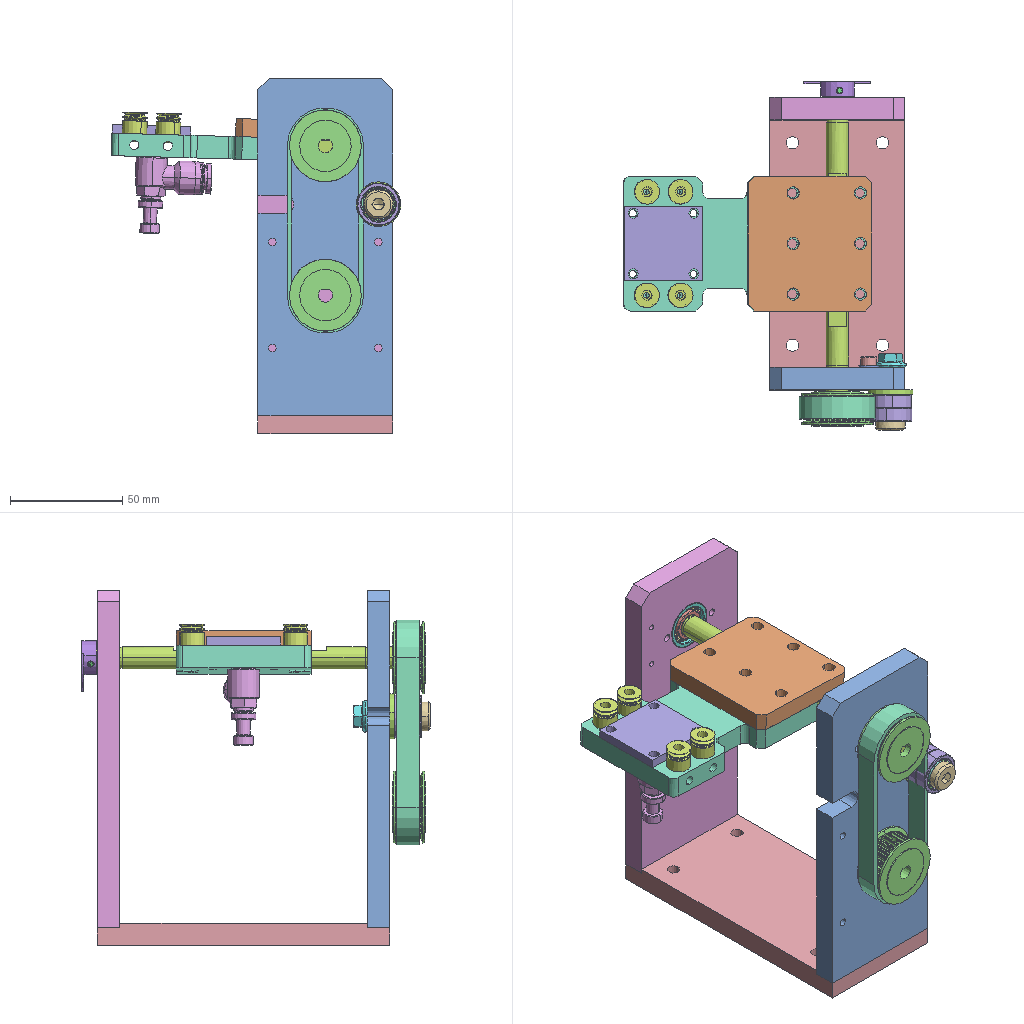Assembly | SolidWorks | 38 different items | 46 placed | box 129 x 155 x 158 mm
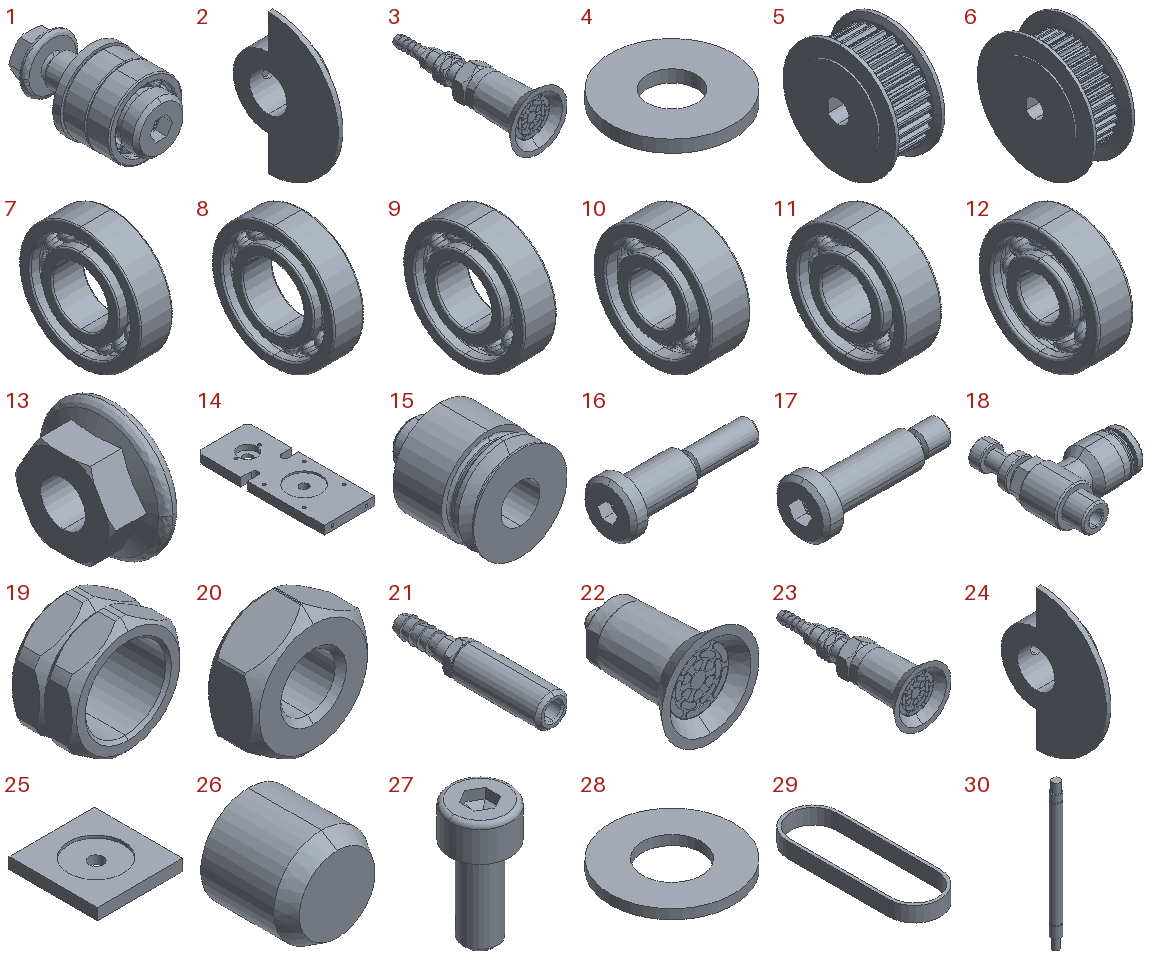Parts list (item | name | quantity | parent item | size | volume | features):
1 | (subassembly) | x1 | - | 20 x 34 x 20 mm | 4809 mm3 | -
2 | (subassembly) | x1 | - | 6.5 x 22.5 x 30 mm | 1090 mm3 | -
3 | (subassembly) | x1 | - | 26 x 64.9 x 26 mm | 7528 mm3 | -
4 | - | x1 | in 1 | 20 x 20 x 2 mm | 527.788 mm3 | features Extrusion 1
5 | - | x2 | - | 15 x 32 x 32 mm | 8293 mm3 | features BaseBody 1
6 | - | x1 | - | 15 x 40 x 40 mm | 11573 mm3 | features BaseBody 1
7 | - | x1 | - | 3.5 x 13 x 13 mm | 272.002 mm3 | features BaseBody 16
8 | - | x1 | - | 4 x 16 x 16 mm | 445.743 mm3 | features BaseBody 17
9 | - | x2 | - | 6 x 22 x 22 mm | 1331 mm3 | features BaseBody 15
10 | - | x1 | - | 5 x 15 x 15 mm | 545.791 mm3 | features BaseBody 14
11 | - | x2 | in 1 | 6 x 19 x 19 mm | 1020 mm3 | features BaseBody 14
12 | - | x1 | - | 9 x 30 x 30 mm | 4206 mm3 | features BaseBody 12
13 | - | x1 | in 1 | 6 x 14.2 x 14.2 mm | 511.274 mm3 | features BaseBody 1
14 | - | x1 | - | 60 x 150 x 10 mm | 80933 mm3 | features Cut 4, HoleWzd 3, Chamfer 1, Extrusion 1, ICE 1, MirrorPattern 1
15 | - | x4 | - | 11 x 13 x 11 mm | 720.123 mm3 | features BaseBody 1
16 | - | x1 | - | 24.5 x 9 x 9 mm | 556.102 mm3 | features BaseBody 1
17 | - | x1 | in 1 | 34 x 13 x 13 mm | 1729 mm3 | features BaseBody 1
18 | - | x1 | - | 33.5 x 41.5 x 15 mm | 5374 mm3 | features BaseBody 1
19 | - | x1 | - | 10 x 6 x 11 mm | 236.508 mm3 | features BaseBody 1
20 | - | x1 | - | 14 x 6.2 x 16 mm | 801.096 mm3 | features BaseBody 1
21 | - | x1 | - | 8 x 38 x 8 mm | 1345 mm3 | features BaseBody 1
22 | - | x1 | - | 26 x 31.5 x 26 mm | 5146 mm3 | features BaseBody 1
23 | - | x1 | - | 26 x 64.9 x 26 mm | 7528 mm3 | features BaseBody 4
24 | - | x1 | in 2 | 6.5 x 22.5 x 30 mm | 1036 mm3 | features BaseBody 1
25 | - | x1 | - | 60 x 62 x 8 mm | 26960 mm3 | features Cut 2, Extrusion 1
26 | - | x3 | in 2 | 3 x 3 x 3 mm | 17.925 mm3 | features BaseBody 1
27 | - | x1 | - | 7 x 7 x 14 mm | 265.768 mm3 | features Chamfer 2, Fillet 2, ICE 2, Extrusion 1, RefAxis 1
28 | - | x1 | - | 9 x 9 x 0.7 mm | 34.367 mm3 | features Extrusion 1, RefAxis 1
29 | - | x1 | - | 33.89 x 100.315 x 10 mm | 4661 mm3 | features BeltProfileFeature 1, ExtruThin 1
30 | - | x1 | - | 10 x 10 x 150 mm | 10228 mm3 | features ICE 4, LibraryFeature 2, RevCut 2, Cut 1, Extrusion 1
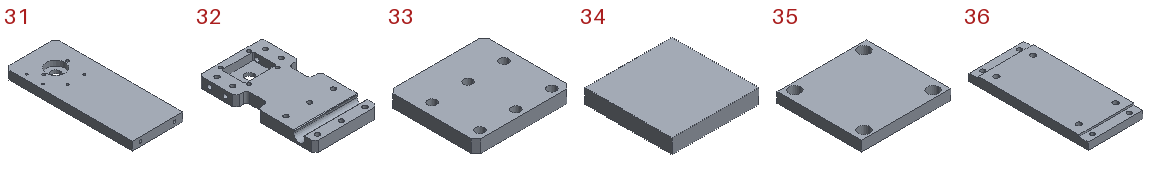31 | - | x1 | - | 60 x 150 x 10 mm | 86519 mm3 | features HoleWzd 3, ICE 2, Chamfer 1, Extrusion 1
32 | - | x1 | - | 60 x 110 x 10 mm | 50711 mm3 | features HoleWzd 5, Chamfer 2, Cut 2, Fillet 2, Extrusion 1, ICE 1, MirrorPattern 1
33 | - | x1 | - | 60 x 55 x 8 mm | 25116 mm3 | features Chamfer 1, Extrusion 1, HoleWzd 1
34 | - | x1 | - | 60 x 60 x 10 mm | 36000 mm3 | features Extrusion 1
35 | - | x1 | - | 35 x 33 x 4 mm | 4366 mm3 | features Extrusion 1, HoleWzd 1
36 | - | x1 | - | 60 x 130 x 10 mm | 73508 mm3 | features HoleWzd 2, Extrusion 1, ICE 1
37 | EE-SX672(with Wiring Terminal) | x1 | - | - | - | -
38 | Leadshine57HS09 | x1 | - | - | - | -
Mates (type | each side: item.copy, entity, surface, feature):
In the top assembly
Coincident | 36.1 face plane Cut-Extrude1 | 14.1 face plane Boss-Extrude1
Coincident | 36.1 face plane Boss-Extrude1 | 14.1 face plane Boss-Extrude1 | 2 times
DistanceDim | 5.1 face plane Input 1 | 14.1 face plane Boss-Extrude1
Concentric | 14.1 face cylinder Cut-Extrude7 | 9.1 face cylinder Input 10
Coincident | 14.1 face plane Cut-Extrude7 | 9.1 face plane Input 10
Concentric | 14.1 face cylinder Cut-Extrude8 | 30.1 face cylinder Boss-Extrude1
Coincident | 36.1 face plane Cut-Extrude1 | 31.1 face plane Boss-Extrude1 | 2 times
Coincident | 36.1 face plane Boss-Extrude1 | 31.1 face plane Boss-Extrude1
Concentric | 31.1 face cylinder Cut-Extrude1 | 9.2 face cylinder Input 10
Coincident | 31.1 face plane Boss-Extrude1 | 9.2 face plane Input 10
Concentric | 30.1 face cylinder Boss-Extrude1 | 32.1 face cylinder Cut-Extrude1
Width | 31.1 face plane Boss-Extrude1 | 14.1 face plane Boss-Extrude1 | 32.1 face plane Boss-Extrude1 | 32.1 face plane Boss-Extrude1
Coincident | 32.1 face plane Boss-Extrude1 | 33.1 face plane Boss-Extrude1 | 2 times
Width | 33.1 face plane Boss-Extrude1 | 33.1 face plane Boss-Extrude1 | 32.1 face plane Boss-Extrude1 | 32.1 face plane Boss-Extrude1
Concentric | 30.1 face cylinder Cut-Extrude2 | 5.2 face cylinder Input 1
Coincident | 5.1 face plane Input 1 | 5.2 face plane Input 1
BeltDim | 5.2 face cylinder Input 1 | 5.1 face cylinder Input 1
Coincident | 14.1 face plane Boss-Extrude1 | 28.1 plane
Coincident | 27.1 plane | 28.1 plane
Concentric | 14.1 face cylinder M4 Tapped Hole2 | 27.1 axis
Coincident | 27.1 axis | 28.1 axis
Parallel | 30.1 face plane Cut-Extrude1 | 32.1 face plane Boss-Extrude1
Concentric | 30.1 face cylinder Boss-Extrude1 | 24.1 face cylinder Input 1
Coincident | 30.1 face plane Boss-Extrude1 | 24.1 face plane Input 1
Concentric | 32.1 face cylinder M5 Tapped Hole2 | 15.1 face cylinder Input 1
Coincident | 32.1 face plane Boss-Extrude1 | 15.1 face plane Input 1
Coincident | 32.1 face plane Boss-Extrude1 | 15.2 face plane Input 1
Concentric | 32.1 face cylinder M5 Tapped Hole2 | 15.2 face cylinder Input 1
Coincident | 32.1 face plane Boss-Extrude1 | 15.3 face plane Input 1
Concentric | 32.1 face cylinder M5 Tapped Hole2 | 15.3 face cylinder Input 1
Coincident | 32.1 face plane Boss-Extrude1 | 15.4 face plane Input 1
Concentric | 32.1 face cylinder M5 Tapped Hole2 | 15.4 face cylinder Input 1
Coincident | 32.1 face plane Boss-Extrude1 | 35.1 face plane Boss-Extrude1 | 2 times
Width | 32.1 face plane Boss-Extrude1 | 32.1 face plane Boss-Extrude1 | 35.1 face plane Boss-Extrude1 | 35.1 face plane Boss-Extrude1
Concentric | 32.1 face cylinder G1/8 Tapped Hole1 | 18.1 face cylinder Input 1
Coincident | 32.1 face plane Boss-Extrude1 | 18.1 face plane Input 1
Parallel | 30.1 face plane Cut-Extrude3 | 5.2 face plane Input 1
Coincident | 14.1 face plane Boss-Extrude1 | 4.1 face plane Boss-Extrude1
Coincident | 14.1 face plane Boss-Extrude1 | 13.1 face plane Input 1
Width | 14.1 face plane Cut-Extrude9 | 14.1 face plane Cut-Extrude9 | 17.1 face cylinder Input 1
Parallel | 36.1 face plane Boss-Extrude1 | 17.1 plane
In subassembly 1
Concentric | 17.2 face cylinder Input 1 | 4.2 face cylinder Boss-Extrude1
Coincident | 11.1 face plane Input 4 | 4.2 face plane Boss-Extrude1
Concentric | 17.2 face cylinder Input 1 | 11.2 face cylinder Input 2
Coincident | 17.2 face plane Input 1 | 11.2 face plane Input 2
Coincident | 11.2 face plane Input 4 | 11.1 face plane Input 4
Concentric | 17.2 face cylinder Input 1 | 11.1 face cylinder Input 2
Concentric | 17.2 face cylinder Input 1 | 13.2 face cylinder Input 1